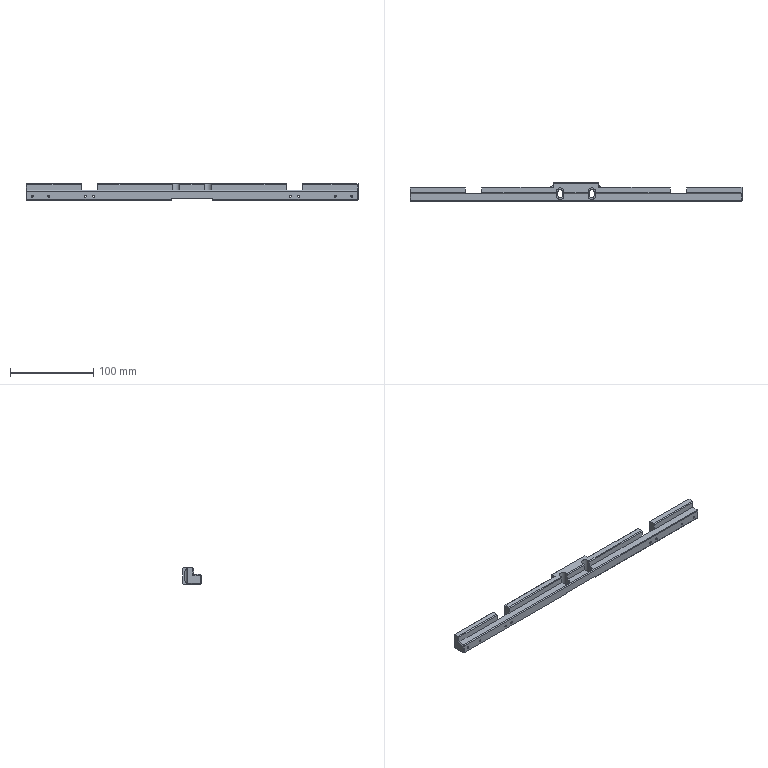Part | NX | 1 solid | 97 faces | box 400 x 22 x 20 mm | volume 99969 mm3 | plane 75 | cylinder 18 | cone 4 | commonest cylinder face diameters 2.5 x8 5.4 x4 9 x4 6 x2